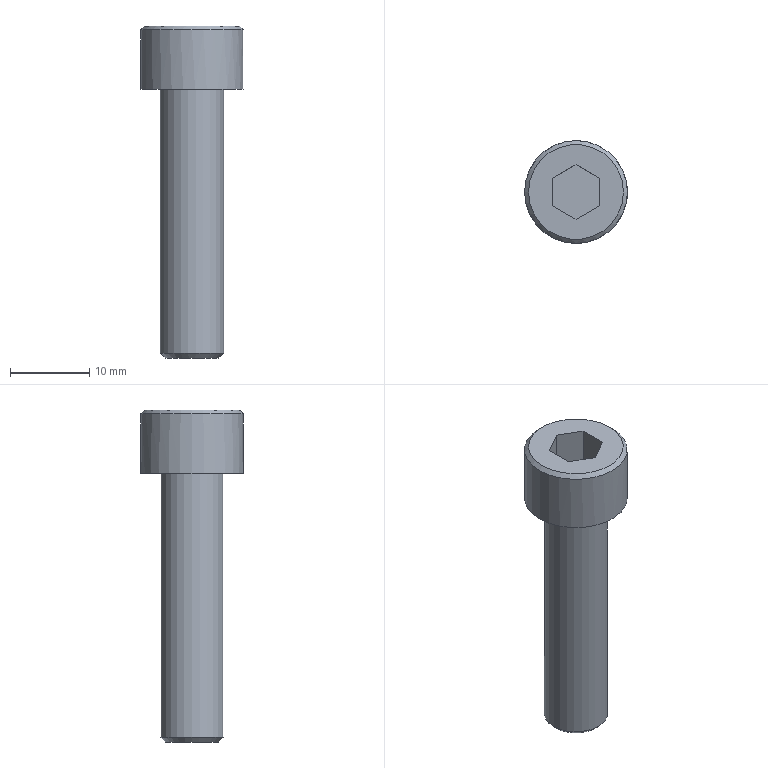Part | STEP file | gslz 2016.10.28-6_id910_x_t | 1 solid | 14 faces | box 13 x 13 x 42 mm | volume 2606 mm3 | plane 10 | cylinder 2 | cone 2 | commonest cylinder face diameters 8 x1 13 x1
STEP:
#1=CARTESIAN_POINT('',(-44.5,249.,27.));
#2=VERTEX_POINT('',#1);
#3=CARTESIAN_POINT('',(-50.5,249.,27.));
#4=DIRECTION('',(0.,0.,1.));
#5=DIRECTION('',(1.,0.,0.));
#6=AXIS2_PLACEMENT_3D('',#3,#4,#5);
#7=CIRCLE('',#6,6.);
#8=EDGE_CURVE('',#2,#2,#7,.T.);
#9=ORIENTED_EDGE('',*,*,#8,.T.);
#10=EDGE_LOOP('',(#9));
#11=FACE_BOUND('',#10,.T.);
#12=CARTESIAN_POINT('',(-53.5,250.732,27.));
#13=VERTEX_POINT('',#12);
#14=CARTESIAN_POINT('',(-53.5,247.268,27.));
#15=VERTEX_POINT('',#14);
#16=CARTESIAN_POINT('',(-53.5,250.732,27.));
#17=DIRECTION('',(0.,-1.,0.));
#18=VECTOR('',#17,1.);
#19=LINE('',#16,#18);
#20=EDGE_CURVE('',#13,#15,#19,.T.);
#21=ORIENTED_EDGE('',*,*,#20,.F.);
#22=CARTESIAN_POINT('',(-50.5,252.464,27.));
#23=VERTEX_POINT('',#22);
#24=CARTESIAN_POINT('',(-50.5,252.464,27.));
#25=DIRECTION('',(-0.866,-0.5,0.));
#26=VECTOR('',#25,1.);
#27=LINE('',#24,#26);
#28=EDGE_CURVE('',#23,#13,#27,.T.);
#29=ORIENTED_EDGE('',*,*,#28,.F.);
#30=CARTESIAN_POINT('',(-47.5,250.732,27.));
#31=VERTEX_POINT('',#30);
#32=CARTESIAN_POINT('',(-47.5,250.732,27.));
#33=DIRECTION('',(-0.866,0.5,0.));
#34=VECTOR('',#33,1.);
#35=LINE('',#32,#34);
#36=EDGE_CURVE('',#31,#23,#35,.T.);
#37=ORIENTED_EDGE('',*,*,#36,.F.);
#38=CARTESIAN_POINT('',(-47.5,247.268,27.));
#39=VERTEX_POINT('',#38);
#40=CARTESIAN_POINT('',(-47.5,247.268,27.));
#41=DIRECTION('',(0.,1.,0.));
#42=VECTOR('',#41,1.);
#43=LINE('',#40,#42);
#44=EDGE_CURVE('',#39,#31,#43,.T.);
#45=ORIENTED_EDGE('',*,*,#44,.F.);
#46=CARTESIAN_POINT('',(-50.5,245.536,27.));
#47=VERTEX_POINT('',#46);
#48=CARTESIAN_POINT('',(-50.5,245.536,27.));
#49=DIRECTION('',(0.866,0.5,0.));
#50=VECTOR('',#49,1.);
#51=LINE('',#48,#50);
#52=EDGE_CURVE('',#47,#39,#51,.T.);
#53=ORIENTED_EDGE('',*,*,#52,.F.);
#54=CARTESIAN_POINT('',(-53.5,247.268,27.));
#55=DIRECTION('',(0.866,-0.5,0.));
#56=VECTOR('',#55,1.);
#57=LINE('',#54,#56);
#58=EDGE_CURVE('',#15,#47,#57,.T.);
#59=ORIENTED_EDGE('',*,*,#58,.F.);
#60=EDGE_LOOP('',(#21,#29,#37,#45,#53,#59));
#61=FACE_BOUND('',#60,.T.);
#62=CARTESIAN_POINT('',(-50.5,249.,27.));
#63=DIRECTION('',(0.,0.,1.));
#64=DIRECTION('',(-1.,0.,0.));
#65=AXIS2_PLACEMENT_3D('',#62,#63,#64);
#66=PLANE('',#65);
#67=ADVANCED_FACE('',(#11,#61),#66,.T.);
#68=CARTESIAN_POINT('',(-53.9,249.,-15.));
#69=VERTEX_POINT('',#68);
#70=CARTESIAN_POINT('',(-50.5,249.,-15.));
#71=DIRECTION('',(0.,0.,-1.));
#72=DIRECTION('',(-1.,0.,0.));
#73=AXIS2_PLACEMENT_3D('',#70,#71,#72);
#74=CIRCLE('',#73,3.4);
#75=EDGE_CURVE('',#69,#69,#74,.T.);
#76=ORIENTED_EDGE('',*,*,#75,.T.);
#77=EDGE_LOOP('',(#76));
#78=FACE_OUTER_BOUND('',#77,.T.);
#79=CARTESIAN_POINT('',(-50.5,249.,-15.));
#80=DIRECTION('',(0.,0.,-1.));
#81=DIRECTION('',(1.,0.,0.));
#82=AXIS2_PLACEMENT_3D('',#79,#80,#81);
#83=PLANE('',#82);
#84=ADVANCED_FACE('',(#78),#83,.T.);
#85=CARTESIAN_POINT('',(-54.5,249.,-14.4));
#86=VERTEX_POINT('',#85);
#87=CARTESIAN_POINT('',(-50.5,249.,-14.4));
#88=DIRECTION('',(0.,0.,1.));
#89=DIRECTION('',(-1.,0.,0.));
#90=AXIS2_PLACEMENT_3D('',#87,#88,#89);
#91=CIRCLE('',#90,4.);
#92=EDGE_CURVE('',#86,#86,#91,.T.);
#93=ORIENTED_EDGE('',*,*,#92,.T.);
#94=EDGE_LOOP('',(#93));
#95=FACE_BOUND('',#94,.T.);
#96=CARTESIAN_POINT('',(-54.5,249.,19.));
#97=VERTEX_POINT('',#96);
#98=CARTESIAN_POINT('',(-50.5,249.,19.));
#99=DIRECTION('',(0.,0.,-1.));
#100=DIRECTION('',(-1.,0.,0.));
#101=AXIS2_PLACEMENT_3D('',#98,#99,#100);
#102=CIRCLE('',#101,4.);
#103=EDGE_CURVE('',#97,#97,#102,.T.);
#104=ORIENTED_EDGE('',*,*,#103,.T.);
#105=EDGE_LOOP('',(#104));
#106=FACE_BOUND('',#105,.T.);
#107=CARTESIAN_POINT('',(-50.5,249.,0.));
#108=DIRECTION('',(0.,0.,-1.));
#109=DIRECTION('',(-1.,0.,0.));
#110=AXIS2_PLACEMENT_3D('',#107,#108,#109);
#111=CYLINDRICAL_SURFACE('',#110,4.);
#112=ADVANCED_FACE('',(#95,#106),#111,.T.);
#113=ORIENTED_EDGE('',*,*,#103,.F.);
#114=EDGE_LOOP('',(#113));
#115=FACE_BOUND('',#114,.T.);
#116=CARTESIAN_POINT('',(-57.,249.,19.));
#117=VERTEX_POINT('',#116);
#118=CARTESIAN_POINT('',(-50.5,249.,19.));
#119=DIRECTION('',(0.,0.,-1.));
#120=DIRECTION('',(-1.,0.,0.));
#121=AXIS2_PLACEMENT_3D('',#118,#119,#120);
#122=CIRCLE('',#121,6.5);
#123=EDGE_CURVE('',#117,#117,#122,.T.);
#124=ORIENTED_EDGE('',*,*,#123,.T.);
#125=EDGE_LOOP('',(#124));
#126=FACE_BOUND('',#125,.T.);
#127=CARTESIAN_POINT('',(-50.5,249.,19.));
#128=DIRECTION('',(0.,0.,-1.));
#129=DIRECTION('',(1.,0.,0.));
#130=AXIS2_PLACEMENT_3D('',#127,#128,#129);
#131=PLANE('',#130);
#132=ADVANCED_FACE('',(#115,#126),#131,.T.);
#133=CARTESIAN_POINT('',(-44.,249.,26.5));
#134=VERTEX_POINT('',#133);
#135=CARTESIAN_POINT('',(-50.5,249.,26.5));
#136=DIRECTION('',(0.,0.,-1.));
#137=DIRECTION('',(1.,0.,0.));
#138=AXIS2_PLACEMENT_3D('',#135,#136,#137);
#139=CIRCLE('',#138,6.5);
#140=EDGE_CURVE('',#134,#134,#139,.T.);
#141=ORIENTED_EDGE('',*,*,#140,.T.);
#142=EDGE_LOOP('',(#141));
#143=FACE_BOUND('',#142,.T.);
#144=ORIENTED_EDGE('',*,*,#123,.F.);
#145=EDGE_LOOP('',(#144));
#146=FACE_BOUND('',#145,.T.);
#147=CARTESIAN_POINT('',(-50.5,249.,30.));
#148=DIRECTION('',(0.,0.,-1.));
#149=DIRECTION('',(-1.,0.,0.));
#150=AXIS2_PLACEMENT_3D('',#147,#148,#149);
#151=CYLINDRICAL_SURFACE('',#150,6.5);
#152=ADVANCED_FACE('',(#143,#146),#151,.T.);
#153=ORIENTED_EDGE('',*,*,#92,.F.);
#154=EDGE_LOOP('',(#153));
#155=FACE_BOUND('',#154,.T.);
#156=ORIENTED_EDGE('',*,*,#75,.F.);
#157=EDGE_LOOP('',(#156));
#158=FACE_BOUND('',#157,.T.);
#159=CARTESIAN_POINT('',(-50.5,249.,-15.));
#160=DIRECTION('',(0.,0.,1.));
#161=DIRECTION('',(1.,0.,0.));
#162=AXIS2_PLACEMENT_3D('',#159,#160,#161);
#163=CONICAL_SURFACE('',#162,3.4,45.);
#164=ADVANCED_FACE('',(#155,#158),#163,.T.);
#165=ORIENTED_EDGE('',*,*,#20,.T.);
#166=CARTESIAN_POINT('',(-53.5,247.268,22.));
#167=VERTEX_POINT('',#166);
#168=CARTESIAN_POINT('',(-53.5,247.268,22.));
#169=DIRECTION('',(0.,0.,-1.));
#170=VECTOR('',#169,1.);
#171=LINE('',#168,#170);
#172=EDGE_CURVE('',#15,#167,#171,.T.);
#173=ORIENTED_EDGE('',*,*,#172,.T.);
#174=CARTESIAN_POINT('',(-53.5,250.732,22.));
#175=VERTEX_POINT('',#174);
#176=CARTESIAN_POINT('',(-53.5,250.732,22.));
#177=DIRECTION('',(0.,1.,0.));
#178=VECTOR('',#177,1.);
#179=LINE('',#176,#178);
#180=EDGE_CURVE('',#167,#175,#179,.T.);
#181=ORIENTED_EDGE('',*,*,#180,.T.);
#182=CARTESIAN_POINT('',(-53.5,250.732,22.));
#183=DIRECTION('',(0.,0.,-1.));
#184=VECTOR('',#183,1.);
#185=LINE('',#182,#184);
#186=EDGE_CURVE('',#13,#175,#185,.T.);
#187=ORIENTED_EDGE('',*,*,#186,.F.);
#188=EDGE_LOOP('',(#165,#173,#181,#187));
#189=FACE_OUTER_BOUND('',#188,.T.);
#190=CARTESIAN_POINT('',(-53.5,250.732,22.));
#191=DIRECTION('',(-1.,0.,0.));
#192=DIRECTION('',(0.,0.,1.));
#193=AXIS2_PLACEMENT_3D('',#190,#191,#192);
#194=PLANE('',#193);
#195=ADVANCED_FACE('',(#189),#194,.F.);
#196=ORIENTED_EDGE('',*,*,#58,.T.);
#197=CARTESIAN_POINT('',(-50.5,245.536,22.));
#198=VERTEX_POINT('',#197);
#199=CARTESIAN_POINT('',(-50.5,245.536,22.));
#200=DIRECTION('',(0.,0.,-1.));
#201=VECTOR('',#200,1.);
#202=LINE('',#199,#201);
#203=EDGE_CURVE('',#47,#198,#202,.T.);
#204=ORIENTED_EDGE('',*,*,#203,.T.);
#205=CARTESIAN_POINT('',(-53.5,247.268,22.));
#206=DIRECTION('',(-0.866,0.5,0.));
#207=VECTOR('',#206,1.);
#208=LINE('',#205,#207);
#209=EDGE_CURVE('',#198,#167,#208,.T.);
#210=ORIENTED_EDGE('',*,*,#209,.T.);
#211=ORIENTED_EDGE('',*,*,#172,.F.);
#212=EDGE_LOOP('',(#196,#204,#210,#211));
#213=FACE_OUTER_BOUND('',#212,.T.);
#214=CARTESIAN_POINT('',(-53.5,247.268,22.));
#215=DIRECTION('',(-0.5,-0.866,0.));
#216=DIRECTION('',(-0.866,0.5,0.));
#217=AXIS2_PLACEMENT_3D('',#214,#215,#216);
#218=PLANE('',#217);
#219=ADVANCED_FACE('',(#213),#218,.F.);
#220=ORIENTED_EDGE('',*,*,#52,.T.);
#221=CARTESIAN_POINT('',(-47.5,247.268,22.));
#222=VERTEX_POINT('',#221);
#223=CARTESIAN_POINT('',(-47.5,247.268,22.));
#224=DIRECTION('',(0.,0.,-1.));
#225=VECTOR('',#224,1.);
#226=LINE('',#223,#225);
#227=EDGE_CURVE('',#39,#222,#226,.T.);
#228=ORIENTED_EDGE('',*,*,#227,.T.);
#229=CARTESIAN_POINT('',(-50.5,245.536,22.));
#230=DIRECTION('',(-0.866,-0.5,0.));
#231=VECTOR('',#230,1.);
#232=LINE('',#229,#231);
#233=EDGE_CURVE('',#222,#198,#232,.T.);
#234=ORIENTED_EDGE('',*,*,#233,.T.);
#235=ORIENTED_EDGE('',*,*,#203,.F.);
#236=EDGE_LOOP('',(#220,#228,#234,#235));
#237=FACE_OUTER_BOUND('',#236,.T.);
#238=CARTESIAN_POINT('',(-50.5,245.536,22.));
#239=DIRECTION('',(0.5,-0.866,0.));
#240=DIRECTION('',(-0.866,-0.5,0.));
#241=AXIS2_PLACEMENT_3D('',#238,#239,#240);
#242=PLANE('',#241);
#243=ADVANCED_FACE('',(#237),#242,.F.);
#244=ORIENTED_EDGE('',*,*,#44,.T.);
#245=CARTESIAN_POINT('',(-47.5,250.732,22.));
#246=VERTEX_POINT('',#245);
#247=CARTESIAN_POINT('',(-47.5,250.732,22.));
#248=DIRECTION('',(0.,0.,-1.));
#249=VECTOR('',#248,1.);
#250=LINE('',#247,#249);
#251=EDGE_CURVE('',#31,#246,#250,.T.);
#252=ORIENTED_EDGE('',*,*,#251,.T.);
#253=CARTESIAN_POINT('',(-47.5,247.268,22.));
#254=DIRECTION('',(0.,-1.,0.));
#255=VECTOR('',#254,1.);
#256=LINE('',#253,#255);
#257=EDGE_CURVE('',#246,#222,#256,.T.);
#258=ORIENTED_EDGE('',*,*,#257,.T.);
#259=ORIENTED_EDGE('',*,*,#227,.F.);
#260=EDGE_LOOP('',(#244,#252,#258,#259));
#261=FACE_OUTER_BOUND('',#260,.T.);
#262=CARTESIAN_POINT('',(-47.5,247.268,22.));
#263=DIRECTION('',(1.,0.,0.));
#264=DIRECTION('',(0.,0.,1.));
#265=AXIS2_PLACEMENT_3D('',#262,#263,#264);
#266=PLANE('',#265);
#267=ADVANCED_FACE('',(#261),#266,.F.);
#268=ORIENTED_EDGE('',*,*,#36,.T.);
#269=CARTESIAN_POINT('',(-50.5,252.464,22.));
#270=VERTEX_POINT('',#269);
#271=CARTESIAN_POINT('',(-50.5,252.464,22.));
#272=DIRECTION('',(0.,0.,-1.));
#273=VECTOR('',#272,1.);
#274=LINE('',#271,#273);
#275=EDGE_CURVE('',#23,#270,#274,.T.);
#276=ORIENTED_EDGE('',*,*,#275,.T.);
#277=CARTESIAN_POINT('',(-47.5,250.732,22.));
#278=DIRECTION('',(0.866,-0.5,0.));
#279=VECTOR('',#278,1.);
#280=LINE('',#277,#279);
#281=EDGE_CURVE('',#270,#246,#280,.T.);
#282=ORIENTED_EDGE('',*,*,#281,.T.);
#283=ORIENTED_EDGE('',*,*,#251,.F.);
#284=EDGE_LOOP('',(#268,#276,#282,#283));
#285=FACE_OUTER_BOUND('',#284,.T.);
#286=CARTESIAN_POINT('',(-47.5,250.732,22.));
#287=DIRECTION('',(0.5,0.866,0.));
#288=DIRECTION('',(0.866,-0.5,0.));
#289=AXIS2_PLACEMENT_3D('',#286,#287,#288);
#290=PLANE('',#289);
#291=ADVANCED_FACE('',(#285),#290,.F.);
#292=ORIENTED_EDGE('',*,*,#28,.T.);
#293=ORIENTED_EDGE('',*,*,#186,.T.);
#294=CARTESIAN_POINT('',(-50.5,252.464,22.));
#295=DIRECTION('',(0.866,0.5,0.));
#296=VECTOR('',#295,1.);
#297=LINE('',#294,#296);
#298=EDGE_CURVE('',#175,#270,#297,.T.);
#299=ORIENTED_EDGE('',*,*,#298,.T.);
#300=ORIENTED_EDGE('',*,*,#275,.F.);
#301=EDGE_LOOP('',(#292,#293,#299,#300));
#302=FACE_OUTER_BOUND('',#301,.T.);
#303=CARTESIAN_POINT('',(-50.5,252.464,22.));
#304=DIRECTION('',(-0.5,0.866,0.));
#305=DIRECTION('',(0.866,0.5,0.));
#306=AXIS2_PLACEMENT_3D('',#303,#304,#305);
#307=PLANE('',#306);
#308=ADVANCED_FACE('',(#302),#307,.F.);
#309=ORIENTED_EDGE('',*,*,#180,.F.);
#310=ORIENTED_EDGE('',*,*,#209,.F.);
#311=ORIENTED_EDGE('',*,*,#233,.F.);
#312=ORIENTED_EDGE('',*,*,#257,.F.);
#313=ORIENTED_EDGE('',*,*,#281,.F.);
#314=ORIENTED_EDGE('',*,*,#298,.F.);
#315=EDGE_LOOP('',(#309,#310,#311,#312,#313,#314));
#316=FACE_OUTER_BOUND('',#315,.T.);
#317=CARTESIAN_POINT('',(-53.5,247.268,22.));
#318=DIRECTION('',(0.,0.,1.));
#319=DIRECTION('',(-1.,0.,0.));
#320=AXIS2_PLACEMENT_3D('',#317,#318,#319);
#321=PLANE('',#320);
#322=ADVANCED_FACE('',(#316),#321,.T.);
#323=ORIENTED_EDGE('',*,*,#8,.F.);
#324=EDGE_LOOP('',(#323));
#325=FACE_BOUND('',#324,.T.);
#326=ORIENTED_EDGE('',*,*,#140,.F.);
#327=EDGE_LOOP('',(#326));
#328=FACE_BOUND('',#327,.T.);
#329=CARTESIAN_POINT('',(-50.5,249.,26.5));
#330=DIRECTION('',(0.,0.,-1.));
#331=DIRECTION('',(-1.,0.,0.));
#332=AXIS2_PLACEMENT_3D('',#329,#330,#331);
#333=CONICAL_SURFACE('',#332,6.5,45.);
#334=ADVANCED_FACE('',(#325,#328),#333,.T.);
#335=CLOSED_SHELL('',(#67,#84,#112,#132,#152,#164,#195,#219,#243,#267,#291,#308,#322,#334));
#336=MANIFOLD_SOLID_BREP('',#335);
#337=(LENGTH_UNIT()NAMED_UNIT(*)SI_UNIT(.MILLI.,.METRE.));
#338=UNCERTAINTY_MEASURE_WITH_UNIT(LENGTH_MEASURE(0.00002),#337,'','');
#339=(NAMED_UNIT(*)PLANE_ANGLE_UNIT()SI_UNIT($,.RADIAN.));
#340=PLANE_ANGLE_MEASURE_WITH_UNIT(PLANE_ANGLE_MEASURE(0.01745),#339);
#341=DIMENSIONAL_EXPONENTS(0.,0.,0.,0.,0.,0.,0.);
#342=(CONVERSION_BASED_UNIT('DEGREE',#340)NAMED_UNIT(#341)PLANE_ANGLE_UNIT());
#343=(NAMED_UNIT(*)SI_UNIT($,.STERADIAN.)SOLID_ANGLE_UNIT());
#344=(GEOMETRIC_REPRESENTATION_CONTEXT(3)GLOBAL_UNCERTAINTY_ASSIGNED_CONTEXT((#338))GLOBAL_UNIT_ASSIGNED_CONTEXT((#337,#342,#343))REPRESENTATION_CONTEXT('',''));
#345=ADVANCED_BREP_SHAPE_REPRESENTATION('',(#336),#344);